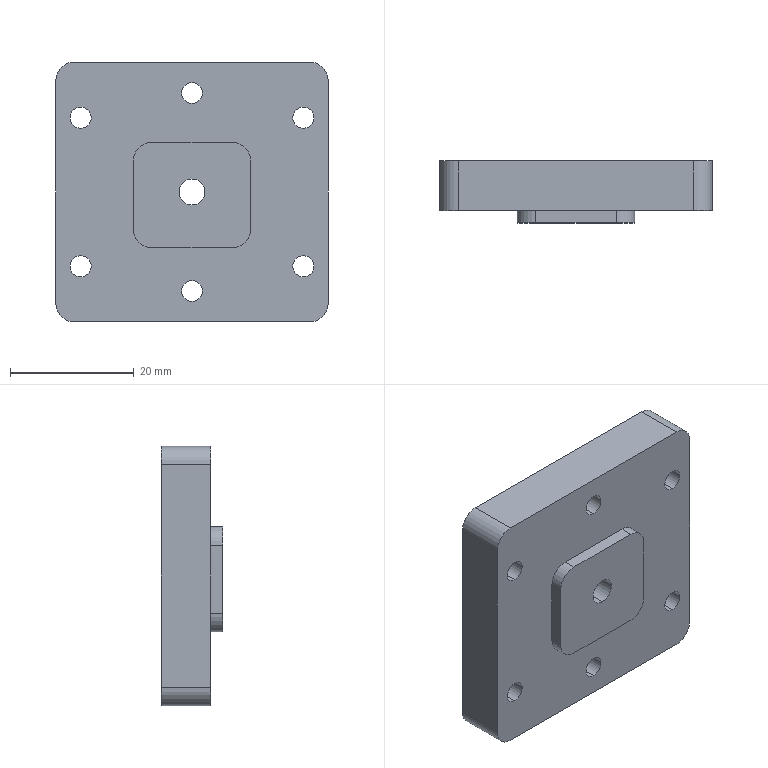Part | STEP file | 10000020483swp000-1 | 1 solid | 51 faces | box 44 x 10 x 42 mm | volume 14387 mm3 | cylinder 34 | plane 17 | commonest cylinder face diameters 6 x20 3.4 x12 4.2 x2
STEP:
#1=CARTESIAN_POINT('',(0.,-2.,-2.1));
#2=VERTEX_POINT('',#1);
#3=CARTESIAN_POINT('',(0.,-2.,2.1));
#4=VERTEX_POINT('',#3);
#5=CARTESIAN_POINT('',(0.,-2.,0.));
#6=DIRECTION('',(0.,1.,0.));
#7=DIRECTION('',(0.,0.,1.));
#8=AXIS2_PLACEMENT_3D('',#5,#6,#7);
#9=CIRCLE('',#8,2.1);
#10=EDGE_CURVE('',#2,#4,#9,.T.);
#11=ORIENTED_EDGE('',*,*,#10,.F.);
#12=CARTESIAN_POINT('',(0.,8.,-2.1));
#13=VERTEX_POINT('',#12);
#14=CARTESIAN_POINT('',(0.,8.,-2.1));
#15=DIRECTION('',(0.,1.,0.));
#16=VECTOR('',#15,1000.);
#17=LINE('',#14,#16);
#18=EDGE_CURVE('',#2,#13,#17,.T.);
#19=ORIENTED_EDGE('',*,*,#18,.T.);
#20=CARTESIAN_POINT('',(0.,8.,2.1));
#21=VERTEX_POINT('',#20);
#22=CARTESIAN_POINT('',(0.,8.,0.));
#23=DIRECTION('',(0.,1.,0.));
#24=DIRECTION('',(0.,0.,1.));
#25=AXIS2_PLACEMENT_3D('',#22,#23,#24);
#26=CIRCLE('',#25,2.1);
#27=EDGE_CURVE('',#13,#21,#26,.T.);
#28=ORIENTED_EDGE('',*,*,#27,.T.);
#29=CARTESIAN_POINT('',(0.,8.,2.1));
#30=DIRECTION('',(0.,1.,0.));
#31=VECTOR('',#30,1000.);
#32=LINE('',#29,#31);
#33=EDGE_CURVE('',#4,#21,#32,.T.);
#34=ORIENTED_EDGE('',*,*,#33,.F.);
#35=EDGE_LOOP('',(#11,#19,#28,#34));
#36=FACE_OUTER_BOUND('',#35,.T.);
#37=CARTESIAN_POINT('',(0.,8.,0.));
#38=DIRECTION('',(0.,1.,0.));
#39=DIRECTION('',(0.,0.,1.));
#40=AXIS2_PLACEMENT_3D('',#37,#38,#39);
#41=CYLINDRICAL_SURFACE('',#40,2.1);
#42=ADVANCED_FACE('',(#36),#41,.F.);
#43=CARTESIAN_POINT('',(0.,4.6,-19.));
#44=VERTEX_POINT('',#43);
#45=CARTESIAN_POINT('',(0.,4.6,-13.));
#46=VERTEX_POINT('',#45);
#47=CARTESIAN_POINT('',(0.,4.6,-16.));
#48=DIRECTION('',(0.,1.,0.));
#49=DIRECTION('',(0.,0.,1.));
#50=AXIS2_PLACEMENT_3D('',#47,#48,#49);
#51=CIRCLE('',#50,3.);
#52=EDGE_CURVE('',#44,#46,#51,.T.);
#53=ORIENTED_EDGE('',*,*,#52,.F.);
#54=CARTESIAN_POINT('',(0.,8.,-19.));
#55=VERTEX_POINT('',#54);
#56=CARTESIAN_POINT('',(0.,8.,-19.));
#57=DIRECTION('',(0.,1.,0.));
#58=VECTOR('',#57,1000.);
#59=LINE('',#56,#58);
#60=EDGE_CURVE('',#44,#55,#59,.T.);
#61=ORIENTED_EDGE('',*,*,#60,.T.);
#62=CARTESIAN_POINT('',(0.,8.,-13.));
#63=VERTEX_POINT('',#62);
#64=CARTESIAN_POINT('',(0.,8.,-16.));
#65=DIRECTION('',(0.,1.,0.));
#66=DIRECTION('',(0.,0.,1.));
#67=AXIS2_PLACEMENT_3D('',#64,#65,#66);
#68=CIRCLE('',#67,3.);
#69=EDGE_CURVE('',#55,#63,#68,.T.);
#70=ORIENTED_EDGE('',*,*,#69,.T.);
#71=CARTESIAN_POINT('',(0.,8.,-13.));
#72=DIRECTION('',(0.,1.,0.));
#73=VECTOR('',#72,1000.);
#74=LINE('',#71,#73);
#75=EDGE_CURVE('',#46,#63,#74,.T.);
#76=ORIENTED_EDGE('',*,*,#75,.F.);
#77=EDGE_LOOP('',(#53,#61,#70,#76));
#78=FACE_OUTER_BOUND('',#77,.T.);
#79=CARTESIAN_POINT('',(0.,8.,-16.));
#80=DIRECTION('',(0.,1.,0.));
#81=DIRECTION('',(0.,0.,1.));
#82=AXIS2_PLACEMENT_3D('',#79,#80,#81);
#83=CYLINDRICAL_SURFACE('',#82,3.);
#84=ADVANCED_FACE('',(#78),#83,.F.);
#85=CARTESIAN_POINT('',(0.,0.,-17.7));
#86=VERTEX_POINT('',#85);
#87=CARTESIAN_POINT('',(0.,0.,-14.3));
#88=VERTEX_POINT('',#87);
#89=CARTESIAN_POINT('',(0.,0.,-16.));
#90=DIRECTION('',(0.,1.,0.));
#91=DIRECTION('',(0.,0.,1.));
#92=AXIS2_PLACEMENT_3D('',#89,#90,#91);
#93=CIRCLE('',#92,1.7);
#94=EDGE_CURVE('',#86,#88,#93,.T.);
#95=ORIENTED_EDGE('',*,*,#94,.F.);
#96=CARTESIAN_POINT('',(0.,4.6,-17.7));
#97=VERTEX_POINT('',#96);
#98=CARTESIAN_POINT('',(0.,8.,-17.7));
#99=DIRECTION('',(0.,1.,0.));
#100=VECTOR('',#99,1000.);
#101=LINE('',#98,#100);
#102=EDGE_CURVE('',#86,#97,#101,.T.);
#103=ORIENTED_EDGE('',*,*,#102,.T.);
#104=CARTESIAN_POINT('',(0.,4.6,-14.3));
#105=VERTEX_POINT('',#104);
#106=CARTESIAN_POINT('',(0.,4.6,-16.));
#107=DIRECTION('',(0.,1.,0.));
#108=DIRECTION('',(0.,0.,1.));
#109=AXIS2_PLACEMENT_3D('',#106,#107,#108);
#110=CIRCLE('',#109,1.7);
#111=EDGE_CURVE('',#97,#105,#110,.T.);
#112=ORIENTED_EDGE('',*,*,#111,.T.);
#113=CARTESIAN_POINT('',(0.,8.,-14.3));
#114=DIRECTION('',(0.,1.,0.));
#115=VECTOR('',#114,1000.);
#116=LINE('',#113,#115);
#117=EDGE_CURVE('',#88,#105,#116,.T.);
#118=ORIENTED_EDGE('',*,*,#117,.F.);
#119=EDGE_LOOP('',(#95,#103,#112,#118));
#120=FACE_OUTER_BOUND('',#119,.T.);
#121=CARTESIAN_POINT('',(0.,8.,-16.));
#122=DIRECTION('',(0.,1.,0.));
#123=DIRECTION('',(0.,0.,1.));
#124=AXIS2_PLACEMENT_3D('',#121,#122,#123);
#125=CYLINDRICAL_SURFACE('',#124,1.7);
#126=ADVANCED_FACE('',(#120),#125,.F.);
#127=CARTESIAN_POINT('',(-18.,4.6,-15.));
#128=VERTEX_POINT('',#127);
#129=CARTESIAN_POINT('',(-18.,4.6,-9.));
#130=VERTEX_POINT('',#129);
#131=CARTESIAN_POINT('',(-18.,4.6,-12.));
#132=DIRECTION('',(0.,1.,0.));
#133=DIRECTION('',(0.,0.,1.));
#134=AXIS2_PLACEMENT_3D('',#131,#132,#133);
#135=CIRCLE('',#134,3.);
#136=EDGE_CURVE('',#128,#130,#135,.T.);
#137=ORIENTED_EDGE('',*,*,#136,.F.);
#138=CARTESIAN_POINT('',(-18.,8.,-15.));
#139=VERTEX_POINT('',#138);
#140=CARTESIAN_POINT('',(-18.,8.,-15.));
#141=DIRECTION('',(0.,1.,0.));
#142=VECTOR('',#141,1000.);
#143=LINE('',#140,#142);
#144=EDGE_CURVE('',#128,#139,#143,.T.);
#145=ORIENTED_EDGE('',*,*,#144,.T.);
#146=CARTESIAN_POINT('',(-18.,8.,-9.));
#147=VERTEX_POINT('',#146);
#148=CARTESIAN_POINT('',(-18.,8.,-12.));
#149=DIRECTION('',(0.,1.,0.));
#150=DIRECTION('',(0.,0.,1.));
#151=AXIS2_PLACEMENT_3D('',#148,#149,#150);
#152=CIRCLE('',#151,3.);
#153=EDGE_CURVE('',#139,#147,#152,.T.);
#154=ORIENTED_EDGE('',*,*,#153,.T.);
#155=CARTESIAN_POINT('',(-18.,8.,-9.));
#156=DIRECTION('',(0.,1.,0.));
#157=VECTOR('',#156,1000.);
#158=LINE('',#155,#157);
#159=EDGE_CURVE('',#130,#147,#158,.T.);
#160=ORIENTED_EDGE('',*,*,#159,.F.);
#161=EDGE_LOOP('',(#137,#145,#154,#160));
#162=FACE_OUTER_BOUND('',#161,.T.);
#163=CARTESIAN_POINT('',(-18.,8.,-12.));
#164=DIRECTION('',(0.,1.,0.));
#165=DIRECTION('',(0.,0.,1.));
#166=AXIS2_PLACEMENT_3D('',#163,#164,#165);
#167=CYLINDRICAL_SURFACE('',#166,3.);
#168=ADVANCED_FACE('',(#162),#167,.F.);
#169=CARTESIAN_POINT('',(-18.,0.,-13.7));
#170=VERTEX_POINT('',#169);
#171=CARTESIAN_POINT('',(-18.,0.,-10.3));
#172=VERTEX_POINT('',#171);
#173=CARTESIAN_POINT('',(-18.,0.,-12.));
#174=DIRECTION('',(0.,1.,0.));
#175=DIRECTION('',(0.,0.,1.));
#176=AXIS2_PLACEMENT_3D('',#173,#174,#175);
#177=CIRCLE('',#176,1.7);
#178=EDGE_CURVE('',#170,#172,#177,.T.);
#179=ORIENTED_EDGE('',*,*,#178,.F.);
#180=CARTESIAN_POINT('',(-18.,4.6,-13.7));
#181=VERTEX_POINT('',#180);
#182=CARTESIAN_POINT('',(-18.,8.,-13.7));
#183=DIRECTION('',(0.,1.,0.));
#184=VECTOR('',#183,1000.);
#185=LINE('',#182,#184);
#186=EDGE_CURVE('',#170,#181,#185,.T.);
#187=ORIENTED_EDGE('',*,*,#186,.T.);
#188=CARTESIAN_POINT('',(-18.,4.6,-10.3));
#189=VERTEX_POINT('',#188);
#190=CARTESIAN_POINT('',(-18.,4.6,-12.));
#191=DIRECTION('',(0.,1.,0.));
#192=DIRECTION('',(0.,0.,1.));
#193=AXIS2_PLACEMENT_3D('',#190,#191,#192);
#194=CIRCLE('',#193,1.7);
#195=EDGE_CURVE('',#181,#189,#194,.T.);
#196=ORIENTED_EDGE('',*,*,#195,.T.);
#197=CARTESIAN_POINT('',(-18.,8.,-10.3));
#198=DIRECTION('',(0.,1.,0.));
#199=VECTOR('',#198,1000.);
#200=LINE('',#197,#199);
#201=EDGE_CURVE('',#172,#189,#200,.T.);
#202=ORIENTED_EDGE('',*,*,#201,.F.);
#203=EDGE_LOOP('',(#179,#187,#196,#202));
#204=FACE_OUTER_BOUND('',#203,.T.);
#205=CARTESIAN_POINT('',(-18.,8.,-12.));
#206=DIRECTION('',(0.,1.,0.));
#207=DIRECTION('',(0.,0.,1.));
#208=AXIS2_PLACEMENT_3D('',#205,#206,#207);
#209=CYLINDRICAL_SURFACE('',#208,1.7);
#210=ADVANCED_FACE('',(#204),#209,.F.);
#211=CARTESIAN_POINT('',(-18.,4.6,9.));
#212=VERTEX_POINT('',#211);
#213=CARTESIAN_POINT('',(-18.,4.6,15.));
#214=VERTEX_POINT('',#213);
#215=CARTESIAN_POINT('',(-18.,4.6,12.));
#216=DIRECTION('',(0.,1.,0.));
#217=DIRECTION('',(0.,0.,1.));
#218=AXIS2_PLACEMENT_3D('',#215,#216,#217);
#219=CIRCLE('',#218,3.);
#220=EDGE_CURVE('',#212,#214,#219,.T.);
#221=ORIENTED_EDGE('',*,*,#220,.F.);
#222=CARTESIAN_POINT('',(-18.,8.,9.));
#223=VERTEX_POINT('',#222);
#224=CARTESIAN_POINT('',(-18.,8.,9.));
#225=DIRECTION('',(0.,1.,0.));
#226=VECTOR('',#225,1000.);
#227=LINE('',#224,#226);
#228=EDGE_CURVE('',#212,#223,#227,.T.);
#229=ORIENTED_EDGE('',*,*,#228,.T.);
#230=CARTESIAN_POINT('',(-18.,8.,15.));
#231=VERTEX_POINT('',#230);
#232=CARTESIAN_POINT('',(-18.,8.,12.));
#233=DIRECTION('',(0.,1.,0.));
#234=DIRECTION('',(0.,0.,1.));
#235=AXIS2_PLACEMENT_3D('',#232,#233,#234);
#236=CIRCLE('',#235,3.);
#237=EDGE_CURVE('',#223,#231,#236,.T.);
#238=ORIENTED_EDGE('',*,*,#237,.T.);
#239=CARTESIAN_POINT('',(-18.,8.,15.));
#240=DIRECTION('',(0.,1.,0.));
#241=VECTOR('',#240,1000.);
#242=LINE('',#239,#241);
#243=EDGE_CURVE('',#214,#231,#242,.T.);
#244=ORIENTED_EDGE('',*,*,#243,.F.);
#245=EDGE_LOOP('',(#221,#229,#238,#244));
#246=FACE_OUTER_BOUND('',#245,.T.);
#247=CARTESIAN_POINT('',(-18.,8.,12.));
#248=DIRECTION('',(0.,1.,0.));
#249=DIRECTION('',(0.,0.,1.));
#250=AXIS2_PLACEMENT_3D('',#247,#248,#249);
#251=CYLINDRICAL_SURFACE('',#250,3.);
#252=ADVANCED_FACE('',(#246),#251,.F.);
#253=CARTESIAN_POINT('',(-18.,0.,10.3));
#254=VERTEX_POINT('',#253);
#255=CARTESIAN_POINT('',(-18.,0.,13.7));
#256=VERTEX_POINT('',#255);
#257=CARTESIAN_POINT('',(-18.,0.,12.));
#258=DIRECTION('',(0.,1.,0.));
#259=DIRECTION('',(0.,0.,1.));
#260=AXIS2_PLACEMENT_3D('',#257,#258,#259);
#261=CIRCLE('',#260,1.7);
#262=EDGE_CURVE('',#254,#256,#261,.T.);
#263=ORIENTED_EDGE('',*,*,#262,.F.);
#264=CARTESIAN_POINT('',(-18.,4.6,10.3));
#265=VERTEX_POINT('',#264);
#266=CARTESIAN_POINT('',(-18.,8.,10.3));
#267=DIRECTION('',(0.,1.,0.));
#268=VECTOR('',#267,1000.);
#269=LINE('',#266,#268);
#270=EDGE_CURVE('',#254,#265,#269,.T.);
#271=ORIENTED_EDGE('',*,*,#270,.T.);
#272=CARTESIAN_POINT('',(-18.,4.6,13.7));
#273=VERTEX_POINT('',#272);
#274=CARTESIAN_POINT('',(-18.,4.6,12.));
#275=DIRECTION('',(0.,1.,0.));
#276=DIRECTION('',(0.,0.,1.));
#277=AXIS2_PLACEMENT_3D('',#274,#275,#276);
#278=CIRCLE('',#277,1.7);
#279=EDGE_CURVE('',#265,#273,#278,.T.);
#280=ORIENTED_EDGE('',*,*,#279,.T.);
#281=CARTESIAN_POINT('',(-18.,8.,13.7));
#282=DIRECTION('',(0.,1.,0.));
#283=VECTOR('',#282,1000.);
#284=LINE('',#281,#283);
#285=EDGE_CURVE('',#256,#273,#284,.T.);
#286=ORIENTED_EDGE('',*,*,#285,.F.);
#287=EDGE_LOOP('',(#263,#271,#280,#286));
#288=FACE_OUTER_BOUND('',#287,.T.);
#289=CARTESIAN_POINT('',(-18.,8.,12.));
#290=DIRECTION('',(0.,1.,0.));
#291=DIRECTION('',(0.,0.,1.));
#292=AXIS2_PLACEMENT_3D('',#289,#290,#291);
#293=CYLINDRICAL_SURFACE('',#292,1.7);
#294=ADVANCED_FACE('',(#288),#293,.F.);
#295=CARTESIAN_POINT('',(0.,4.6,13.));
#296=VERTEX_POINT('',#295);
#297=CARTESIAN_POINT('',(0.,4.6,19.));
#298=VERTEX_POINT('',#297);
#299=CARTESIAN_POINT('',(0.,4.6,16.));
#300=DIRECTION('',(0.,1.,0.));
#301=DIRECTION('',(0.,0.,1.));
#302=AXIS2_PLACEMENT_3D('',#299,#300,#301);
#303=CIRCLE('',#302,3.);
#304=EDGE_CURVE('',#296,#298,#303,.T.);
#305=ORIENTED_EDGE('',*,*,#304,.F.);
#306=CARTESIAN_POINT('',(0.,8.,13.));
#307=VERTEX_POINT('',#306);
#308=CARTESIAN_POINT('',(0.,8.,13.));
#309=DIRECTION('',(0.,1.,0.));
#310=VECTOR('',#309,1000.);
#311=LINE('',#308,#310);
#312=EDGE_CURVE('',#296,#307,#311,.T.);
#313=ORIENTED_EDGE('',*,*,#312,.T.);
#314=CARTESIAN_POINT('',(0.,8.,19.));
#315=VERTEX_POINT('',#314);
#316=CARTESIAN_POINT('',(0.,8.,16.));
#317=DIRECTION('',(0.,1.,0.));
#318=DIRECTION('',(0.,0.,1.));
#319=AXIS2_PLACEMENT_3D('',#316,#317,#318);
#320=CIRCLE('',#319,3.);
#321=EDGE_CURVE('',#307,#315,#320,.T.);
#322=ORIENTED_EDGE('',*,*,#321,.T.);
#323=CARTESIAN_POINT('',(0.,8.,19.));
#324=DIRECTION('',(0.,1.,0.));
#325=VECTOR('',#324,1000.);
#326=LINE('',#323,#325);
#327=EDGE_CURVE('',#298,#315,#326,.T.);
#328=ORIENTED_EDGE('',*,*,#327,.F.);
#329=EDGE_LOOP('',(#305,#313,#322,#328));
#330=FACE_OUTER_BOUND('',#329,.T.);
#331=CARTESIAN_POINT('',(0.,8.,16.));
#332=DIRECTION('',(0.,1.,0.));
#333=DIRECTION('',(0.,0.,1.));
#334=AXIS2_PLACEMENT_3D('',#331,#332,#333);
#335=CYLINDRICAL_SURFACE('',#334,3.);
#336=ADVANCED_FACE('',(#330),#335,.F.);
#337=CARTESIAN_POINT('',(0.,0.,14.3));
#338=VERTEX_POINT('',#337);
#339=CARTESIAN_POINT('',(0.,0.,17.7));
#340=VERTEX_POINT('',#339);
#341=CARTESIAN_POINT('',(0.,0.,16.));
#342=DIRECTION('',(0.,1.,0.));
#343=DIRECTION('',(0.,0.,1.));
#344=AXIS2_PLACEMENT_3D('',#341,#342,#343);
#345=CIRCLE('',#344,1.7);
#346=EDGE_CURVE('',#338,#340,#345,.T.);
#347=ORIENTED_EDGE('',*,*,#346,.F.);
#348=CARTESIAN_POINT('',(0.,4.6,14.3));
#349=VERTEX_POINT('',#348);
#350=CARTESIAN_POINT('',(0.,8.,14.3));
#351=DIRECTION('',(0.,1.,0.));
#352=VECTOR('',#351,1000.);
#353=LINE('',#350,#352);
#354=EDGE_CURVE('',#338,#349,#353,.T.);
#355=ORIENTED_EDGE('',*,*,#354,.T.);
#356=CARTESIAN_POINT('',(0.,4.6,17.7));
#357=VERTEX_POINT('',#356);
#358=CARTESIAN_POINT('',(0.,4.6,16.));
#359=DIRECTION('',(0.,1.,0.));
#360=DIRECTION('',(0.,0.,1.));
#361=AXIS2_PLACEMENT_3D('',#358,#359,#360);
#362=CIRCLE('',#361,1.7);
#363=EDGE_CURVE('',#349,#357,#362,.T.);
#364=ORIENTED_EDGE('',*,*,#363,.T.);
#365=CARTESIAN_POINT('',(0.,8.,17.7));
#366=DIRECTION('',(0.,1.,0.));
#367=VECTOR('',#366,1000.);
#368=LINE('',#365,#367);
#369=EDGE_CURVE('',#340,#357,#368,.T.);
#370=ORIENTED_EDGE('',*,*,#369,.F.);
#371=EDGE_LOOP('',(#347,#355,#364,#370));
#372=FACE_OUTER_BOUND('',#371,.T.);
#373=CARTESIAN_POINT('',(0.,8.,16.));
#374=DIRECTION('',(0.,1.,0.));
#375=DIRECTION('',(0.,0.,1.));
#376=AXIS2_PLACEMENT_3D('',#373,#374,#375);
#377=CYLINDRICAL_SURFACE('',#376,1.7);
#378=ADVANCED_FACE('',(#372),#377,.F.);
#379=CARTESIAN_POINT('',(18.,4.6,9.));
#380=VERTEX_POINT('',#379);
#381=CARTESIAN_POINT('',(18.,4.6,15.));
#382=VERTEX_POINT('',#381);
#383=CARTESIAN_POINT('',(18.,4.6,12.));
#384=DIRECTION('',(0.,1.,0.));
#385=DIRECTION('',(0.,0.,1.));
#386=AXIS2_PLACEMENT_3D('',#383,#384,#385);
#387=CIRCLE('',#386,3.);
#388=EDGE_CURVE('',#380,#382,#387,.T.);
#389=ORIENTED_EDGE('',*,*,#388,.F.);
#390=CARTESIAN_POINT('',(18.,8.,9.));
#391=VERTEX_POINT('',#390);
#392=CARTESIAN_POINT('',(18.,8.,9.));
#393=DIRECTION('',(0.,1.,0.));
#394=VECTOR('',#393,1000.);
#395=LINE('',#392,#394);
#396=EDGE_CURVE('',#380,#391,#395,.T.);
#397=ORIENTED_EDGE('',*,*,#396,.T.);
#398=CARTESIAN_POINT('',(18.,8.,15.));
#399=VERTEX_POINT('',#398);
#400=CARTESIAN_POINT('',(18.,8.,12.));
#401=DIRECTION('',(0.,1.,0.));
#402=DIRECTION('',(0.,0.,1.));
#403=AXIS2_PLACEMENT_3D('',#400,#401,#402);
#404=CIRCLE('',#403,3.);
#405=EDGE_CURVE('',#391,#399,#404,.T.);
#406=ORIENTED_EDGE('',*,*,#405,.T.);
#407=CARTESIAN_POINT('',(18.,8.,15.));
#408=DIRECTION('',(0.,1.,0.));
#409=VECTOR('',#408,1000.);
#410=LINE('',#407,#409);
#411=EDGE_CURVE('',#382,#399,#410,.T.);
#412=ORIENTED_EDGE('',*,*,#411,.F.);
#413=EDGE_LOOP('',(#389,#397,#406,#412));
#414=FACE_OUTER_BOUND('',#413,.T.);
#415=CARTESIAN_POINT('',(18.,8.,12.));
#416=DIRECTION('',(0.,1.,0.));
#417=DIRECTION('',(0.,0.,1.));
#418=AXIS2_PLACEMENT_3D('',#415,#416,#417);
#419=CYLINDRICAL_SURFACE('',#418,3.);
#420=ADVANCED_FACE('',(#414),#419,.F.);
#421=CARTESIAN_POINT('',(18.,0.,10.3));
#422=VERTEX_POINT('',#421);
#423=CARTESIAN_POINT('',(18.,0.,13.7));
#424=VERTEX_POINT('',#423);
#425=CARTESIAN_POINT('',(18.,0.,12.));
#426=DIRECTION('',(0.,1.,0.));
#427=DIRECTION('',(0.,0.,1.));
#428=AXIS2_PLACEMENT_3D('',#425,#426,#427);
#429=CIRCLE('',#428,1.7);
#430=EDGE_CURVE('',#422,#424,#429,.T.);
#431=ORIENTED_EDGE('',*,*,#430,.F.);
#432=CARTESIAN_POINT('',(18.,4.6,10.3));
#433=VERTEX_POINT('',#432);
#434=CARTESIAN_POINT('',(18.,8.,10.3));
#435=DIRECTION('',(0.,1.,0.));
#436=VECTOR('',#435,1000.);
#437=LINE('',#434,#436);
#438=EDGE_CURVE('',#422,#433,#437,.T.);
#439=ORIENTED_EDGE('',*,*,#438,.T.);
#440=CARTESIAN_POINT('',(18.,4.6,13.7));
#441=VERTEX_POINT('',#440);
#442=CARTESIAN_POINT('',(18.,4.6,12.));
#443=DIRECTION('',(0.,1.,0.));
#444=DIRECTION('',(0.,0.,1.));
#445=AXIS2_PLACEMENT_3D('',#442,#443,#444);
#446=CIRCLE('',#445,1.7);
#447=EDGE_CURVE('',#433,#441,#446,.T.);
#448=ORIENTED_EDGE('',*,*,#447,.T.);
#449=CARTESIAN_POINT('',(18.,8.,13.7));
#450=DIRECTION('',(0.,1.,0.));
#451=VECTOR('',#450,1000.);
#452=LINE('',#449,#451);
#453=EDGE_CURVE('',#424,#441,#452,.T.);
#454=ORIENTED_EDGE('',*,*,#453,.F.);
#455=EDGE_LOOP('',(#431,#439,#448,#454));
#456=FACE_OUTER_BOUND('',#455,.T.);
#457=CARTESIAN_POINT('',(18.,8.,12.));
#458=DIRECTION('',(0.,1.,0.));
#459=DIRECTION('',(0.,0.,1.));
#460=AXIS2_PLACEMENT_3D('',#457,#458,#459);
#461=CYLINDRICAL_SURFACE('',#460,1.7);
#462=ADVANCED_FACE('',(#456),#461,.F.);
#463=CARTESIAN_POINT('',(18.,4.6,-15.));
#464=VERTEX_POINT('',#463);
#465=CARTESIAN_POINT('',(18.,4.6,-9.));
#466=VERTEX_POINT('',#465);
#467=CARTESIAN_POINT('',(18.,4.6,-12.));
#468=DIRECTION('',(0.,1.,0.));
#469=DIRECTION('',(0.,0.,1.));
#470=AXIS2_PLACEMENT_3D('',#467,#468,#469);
#471=CIRCLE('',#470,3.);
#472=EDGE_CURVE('',#464,#466,#471,.T.);
#473=ORIENTED_EDGE('',*,*,#472,.F.);
#474=CARTESIAN_POINT('',(18.,8.,-15.));
#475=VERTEX_POINT('',#474);
#476=CARTESIAN_POINT('',(18.,8.,-15.));
#477=DIRECTION('',(0.,1.,0.));
#478=VECTOR('',#477,1000.);
#479=LINE('',#476,#478);
#480=EDGE_CURVE('',#464,#475,#479,.T.);
#481=ORIENTED_EDGE('',*,*,#480,.T.);
#482=CARTESIAN_POINT('',(18.,8.,-9.));
#483=VERTEX_POINT('',#482);
#484=CARTESIAN_POINT('',(18.,8.,-12.));
#485=DIRECTION('',(0.,1.,0.));
#486=DIRECTION('',(0.,0.,1.));
#487=AXIS2_PLACEMENT_3D('',#484,#485,#486);
#488=CIRCLE('',#487,3.);
#489=EDGE_CURVE('',#475,#483,#488,.T.);
#490=ORIENTED_EDGE('',*,*,#489,.T.);
#491=CARTESIAN_POINT('',(18.,8.,-9.));
#492=DIRECTION('',(0.,1.,0.));
#493=VECTOR('',#492,1000.);
#494=LINE('',#491,#493);
#495=EDGE_CURVE('',#466,#483,#494,.T.);
#496=ORIENTED_EDGE('',*,*,#495,.F.);
#497=EDGE_LOOP('',(#473,#481,#490,#496));
#498=FACE_OUTER_BOUND('',#497,.T.);
#499=CARTESIAN_POINT('',(18.,8.,-12.));
#500=DIRECTION('',(0.,1.,0.));
#501=DIRECTION('',(0.,0.,1.));
#502=AXIS2_PLACEMENT_3D('',#499,#500,#501);
#503=CYLINDRICAL_SURFACE('',#502,3.);
#504=ADVANCED_FACE('',(#498),#503,.F.);
#505=CARTESIAN_POINT('',(18.,0.,-13.7));
#506=VERTEX_POINT('',#505);
#507=CARTESIAN_POINT('',(18.,0.,-10.3));
#508=VERTEX_POINT('',#507);
#509=CARTESIAN_POINT('',(18.,0.,-12.));
#510=DIRECTION('',(0.,1.,0.));
#511=DIRECTION('',(0.,0.,1.));
#512=AXIS2_PLACEMENT_3D('',#509,#510,#511);
#513=CIRCLE('',#512,1.7);
#514=EDGE_CURVE('',#506,#508,#513,.T.);
#515=ORIENTED_EDGE('',*,*,#514,.F.);
#516=CARTESIAN_POINT('',(18.,4.6,-13.7));
#517=VERTEX_POINT('',#516);
#518=CARTESIAN_POINT('',(18.,8.,-13.7));
#519=DIRECTION('',(0.,1.,0.));
#520=VECTOR('',#519,1000.);
#521=LINE('',#518,#520);
#522=EDGE_CURVE('',#506,#517,#521,.T.);
#523=ORIENTED_EDGE('',*,*,#522,.T.);
#524=CARTESIAN_POINT('',(18.,4.6,-10.3));
#525=VERTEX_POINT('',#524);
#526=CARTESIAN_POINT('',(18.,4.6,-12.));
#527=DIRECTION('',(0.,1.,0.));
#528=DIRECTION('',(0.,0.,1.));
#529=AXIS2_PLACEMENT_3D('',#526,#527,#528);
#530=CIRCLE('',#529,1.7);
#531=EDGE_CURVE('',#517,#525,#530,.T.);
#532=ORIENTED_EDGE('',*,*,#531,.T.);
#533=CARTESIAN_POINT('',(18.,8.,-10.3));
#534=DIRECTION('',(0.,1.,0.));
#535=VECTOR('',#534,1000.);
#536=LINE('',#533,#535);
#537=EDGE_CURVE('',#508,#525,#536,.T.);
#538=ORIENTED_EDGE('',*,*,#537,.F.);
#539=EDGE_LOOP('',(#515,#523,#532,#538));
#540=FACE_OUTER_BOUND('',#539,.T.);
#541=CARTESIAN_POINT('',(18.,8.,-12.));
#542=DIRECTION('',(0.,1.,0.));
#543=DIRECTION('',(0.,0.,1.));
#544=AXIS2_PLACEMENT_3D('',#541,#542,#543);
#545=CYLINDRICAL_SURFACE('',#544,1.7);
#546=ADVANCED_FACE('',(#540),#545,.F.);
#547=CARTESIAN_POINT('',(0.,0.,-16.));
#548=DIRECTION('',(0.,1.,0.));
#549=DIRECTION('',(0.,0.,1.));
#550=AXIS2_PLACEMENT_3D('',#547,#548,#549);
#551=CIRCLE('',#550,1.7);
#552=EDGE_CURVE('',#88,#86,#551,.T.);
#553=ORIENTED_EDGE('',*,*,#552,.T.);
#554=ORIENTED_EDGE('',*,*,#94,.T.);
#555=EDGE_LOOP('',(#553,#554));
#556=FACE_BOUND('',#555,.T.);
#557=CARTESIAN_POINT('',(-18.,0.,-12.));
#558=DIRECTION('',(0.,1.,0.));
#559=DIRECTION('',(0.,0.,1.));
#560=AXIS2_PLACEMENT_3D('',#557,#558,#559);
#561=CIRCLE('',#560,1.7);
#562=EDGE_CURVE('',#172,#170,#561,.T.);
#563=ORIENTED_EDGE('',*,*,#562,.T.);
#564=ORIENTED_EDGE('',*,*,#178,.T.);
#565=EDGE_LOOP('',(#563,#564));
#566=FACE_BOUND('',#565,.T.);
#567=CARTESIAN_POINT('',(-18.,0.,12.));
#568=DIRECTION('',(0.,1.,0.));
#569=DIRECTION('',(0.,0.,1.));
#570=AXIS2_PLACEMENT_3D('',#567,#568,#569);
#571=CIRCLE('',#570,1.7);
#572=EDGE_CURVE('',#256,#254,#571,.T.);
#573=ORIENTED_EDGE('',*,*,#572,.T.);
#574=ORIENTED_EDGE('',*,*,#262,.T.);
#575=EDGE_LOOP('',(#573,#574));
#576=FACE_BOUND('',#575,.T.);
#577=CARTESIAN_POINT('',(0.,0.,16.));
#578=DIRECTION('',(0.,1.,0.));
#579=DIRECTION('',(0.,0.,1.));
#580=AXIS2_PLACEMENT_3D('',#577,#578,#579);
#581=CIRCLE('',#580,1.7);
#582=EDGE_CURVE('',#340,#338,#581,.T.);
#583=ORIENTED_EDGE('',*,*,#582,.T.);
#584=ORIENTED_EDGE('',*,*,#346,.T.);
#585=EDGE_LOOP('',(#583,#584));
#586=FACE_BOUND('',#585,.T.);
#587=CARTESIAN_POINT('',(18.,0.,12.));
#588=DIRECTION('',(0.,1.,0.));
#589=DIRECTION('',(0.,0.,1.));
#590=AXIS2_PLACEMENT_3D('',#587,#588,#589);
#591=CIRCLE('',#590,1.7);
#592=EDGE_CURVE('',#424,#422,#591,.T.);
#593=ORIENTED_EDGE('',*,*,#592,.T.);
#594=ORIENTED_EDGE('',*,*,#430,.T.);
#595=EDGE_LOOP('',(#593,#594));
#596=FACE_BOUND('',#595,.T.);
#597=CARTESIAN_POINT('',(18.,0.,-12.));
#598=DIRECTION('',(0.,1.,0.));
#599=DIRECTION('',(0.,0.,1.));
#600=AXIS2_PLACEMENT_3D('',#597,#598,#599);
#601=CIRCLE('',#600,1.7);
#602=EDGE_CURVE('',#508,#506,#601,.T.);
#603=ORIENTED_EDGE('',*,*,#602,.T.);
#604=ORIENTED_EDGE('',*,*,#514,.T.);
#605=EDGE_LOOP('',(#603,#604));
#606=FACE_BOUND('',#605,.T.);
#607=CARTESIAN_POINT('',(22.,0.,18.));
#608=VERTEX_POINT('',#607);
#609=CARTESIAN_POINT('',(22.,0.,-18.));
#610=VERTEX_POINT('',#609);
#611=CARTESIAN_POINT('',(22.,0.,-21.));
#612=DIRECTION('',(0.,0.,-1.));
#613=VECTOR('',#612,1000.);
#614=LINE('',#611,#613);
#615=EDGE_CURVE('',#608,#610,#614,.T.);
#616=ORIENTED_EDGE('',*,*,#615,.F.);
#617=CARTESIAN_POINT('',(19.,0.,21.));
#618=VERTEX_POINT('',#617);
#619=CARTESIAN_POINT('',(19.,0.,18.));
#620=DIRECTION('',(0.,-1.,0.));
#621=DIRECTION('',(0.,0.,1.));
#622=AXIS2_PLACEMENT_3D('',#619,#620,#621);
#623=CIRCLE('',#622,3.);
#624=EDGE_CURVE('',#608,#618,#623,.T.);
#625=ORIENTED_EDGE('',*,*,#624,.T.);
#626=CARTESIAN_POINT('',(-19.,0.,21.));
#627=VERTEX_POINT('',#626);
#628=CARTESIAN_POINT('',(-22.,0.,21.));
#629=DIRECTION('',(1.,0.,0.));
#630=VECTOR('',#629,1000.);
#631=LINE('',#628,#630);
#632=EDGE_CURVE('',#627,#618,#631,.T.);
#633=ORIENTED_EDGE('',*,*,#632,.F.);
#634=CARTESIAN_POINT('',(-22.,0.,18.));
#635=VERTEX_POINT('',#634);
#636=CARTESIAN_POINT('',(-19.,0.,18.));
#637=DIRECTION('',(0.,-1.,0.));
#638=DIRECTION('',(0.,0.,1.));
#639=AXIS2_PLACEMENT_3D('',#636,#637,#638);
#640=CIRCLE('',#639,3.);
#641=EDGE_CURVE('',#627,#635,#640,.T.);
#642=ORIENTED_EDGE('',*,*,#641,.T.);
#643=CARTESIAN_POINT('',(-22.,0.,-18.));
#644=VERTEX_POINT('',#643);
#645=CARTESIAN_POINT('',(-22.,0.,-21.));
#646=DIRECTION('',(0.,0.,1.));
#647=VECTOR('',#646,1000.);
#648=LINE('',#645,#647);
#649=EDGE_CURVE('',#644,#635,#648,.T.);
#650=ORIENTED_EDGE('',*,*,#649,.F.);
#651=CARTESIAN_POINT('',(-19.,0.,-21.));
#652=VERTEX_POINT('',#651);
#653=CARTESIAN_POINT('',(-19.,0.,-18.));
#654=DIRECTION('',(0.,-1.,0.));
#655=DIRECTION('',(0.,0.,1.));
#656=AXIS2_PLACEMENT_3D('',#653,#654,#655);
#657=CIRCLE('',#656,3.);
#658=EDGE_CURVE('',#644,#652,#657,.T.);
#659=ORIENTED_EDGE('',*,*,#658,.T.);
#660=CARTESIAN_POINT('',(19.,0.,-21.));
#661=VERTEX_POINT('',#660);
#662=CARTESIAN_POINT('',(-22.,0.,-21.));
#663=DIRECTION('',(-1.,0.,0.));
#664=VECTOR('',#663,1000.);
#665=LINE('',#662,#664);
#666=EDGE_CURVE('',#661,#652,#665,.T.);
#667=ORIENTED_EDGE('',*,*,#666,.F.);
#668=CARTESIAN_POINT('',(19.,0.,-18.));
#669=DIRECTION('',(0.,-1.,0.));
#670=DIRECTION('',(0.,0.,1.));
#671=AXIS2_PLACEMENT_3D('',#668,#669,#670);
#672=CIRCLE('',#671,3.);
#673=EDGE_CURVE('',#661,#610,#672,.T.);
#674=ORIENTED_EDGE('',*,*,#673,.T.);
#675=EDGE_LOOP('',(#616,#625,#633,#642,#650,#659,#667,#674));
#676=FACE_OUTER_BOUND('',#675,.T.);
#677=CARTESIAN_POINT('',(9.5,0.,-6.));
#678=VERTEX_POINT('',#677);
#679=CARTESIAN_POINT('',(9.5,0.,5.));
#680=VERTEX_POINT('',#679);
#681=CARTESIAN_POINT('',(9.5,0.,8.));
#682=DIRECTION('',(0.,0.,1.));
#683=VECTOR('',#682,1000.);
#684=LINE('',#681,#683);
#685=EDGE_CURVE('',#678,#680,#684,.T.);
#686=ORIENTED_EDGE('',*,*,#685,.F.);
#687=CARTESIAN_POINT('',(6.5,0.,-9.));
#688=VERTEX_POINT('',#687);
#689=CARTESIAN_POINT('',(6.5,0.,-6.));
#690=DIRECTION('',(0.,1.,0.));
#691=DIRECTION('',(0.,0.,1.));
#692=AXIS2_PLACEMENT_3D('',#689,#690,#691);
#693=CIRCLE('',#692,3.);
#694=EDGE_CURVE('',#678,#688,#693,.T.);
#695=ORIENTED_EDGE('',*,*,#694,.T.);
#696=CARTESIAN_POINT('',(-6.5,0.,-9.));
#697=VERTEX_POINT('',#696);
#698=CARTESIAN_POINT('',(-9.5,0.,-9.));
#699=DIRECTION('',(1.,0.,0.));
#700=VECTOR('',#699,1000.);
#701=LINE('',#698,#700);
#702=EDGE_CURVE('',#697,#688,#701,.T.);
#703=ORIENTED_EDGE('',*,*,#702,.F.);
#704=CARTESIAN_POINT('',(-9.5,0.,-6.));
#705=VERTEX_POINT('',#704);
#706=CARTESIAN_POINT('',(-6.5,0.,-6.));
#707=DIRECTION('',(0.,1.,0.));
#708=DIRECTION('',(0.,0.,1.));
#709=AXIS2_PLACEMENT_3D('',#706,#707,#708);
#710=CIRCLE('',#709,3.);
#711=EDGE_CURVE('',#697,#705,#710,.T.);
#712=ORIENTED_EDGE('',*,*,#711,.T.);
#713=CARTESIAN_POINT('',(-9.5,0.,5.));
#714=VERTEX_POINT('',#713);
#715=CARTESIAN_POINT('',(-9.5,0.,8.));
#716=DIRECTION('',(0.,0.,-1.));
#717=VECTOR('',#716,1000.);
#718=LINE('',#715,#717);
#719=EDGE_CURVE('',#714,#705,#718,.T.);
#720=ORIENTED_EDGE('',*,*,#719,.F.);
#721=CARTESIAN_POINT('',(-6.5,0.,8.));
#722=VERTEX_POINT('',#721);
#723=CARTESIAN_POINT('',(-6.5,0.,5.));
#724=DIRECTION('',(0.,1.,0.));
#725=DIRECTION('',(0.,0.,1.));
#726=AXIS2_PLACEMENT_3D('',#723,#724,#725);
#727=CIRCLE('',#726,3.);
#728=EDGE_CURVE('',#714,#722,#727,.T.);
#729=ORIENTED_EDGE('',*,*,#728,.T.);
#730=CARTESIAN_POINT('',(6.5,0.,8.));
#731=VERTEX_POINT('',#730);
#732=CARTESIAN_POINT('',(-9.5,0.,8.));
#733=DIRECTION('',(-1.,0.,0.));
#734=VECTOR('',#733,1000.);
#735=LINE('',#732,#734);
#736=EDGE_CURVE('',#731,#722,#735,.T.);
#737=ORIENTED_EDGE('',*,*,#736,.F.);
#738=CARTESIAN_POINT('',(6.5,0.,5.));
#739=DIRECTION('',(0.,1.,0.));
#740=DIRECTION('',(0.,0.,1.));
#741=AXIS2_PLACEMENT_3D('',#738,#739,#740);
#742=CIRCLE('',#741,3.);
#743=EDGE_CURVE('',#731,#680,#742,.T.);
#744=ORIENTED_EDGE('',*,*,#743,.T.);
#745=EDGE_LOOP('',(#686,#695,#703,#712,#720,#729,#737,#744));
#746=FACE_BOUND('',#745,.T.);
#747=CARTESIAN_POINT('',(0.,0.,0.));
#748=DIRECTION('',(0.,1.,0.));
#749=DIRECTION('',(0.,0.,1.));
#750=AXIS2_PLACEMENT_3D('',#747,#748,#749);
#751=PLANE('',#750);
#752=ADVANCED_FACE('',(#556,#566,#576,#586,#596,#606,#676,#746),#751,.F.);
#753=CARTESIAN_POINT('',(22.,8.,18.));
#754=VERTEX_POINT('',#753);
#755=CARTESIAN_POINT('',(22.,8.,-18.));
#756=VERTEX_POINT('',#755);
#757=CARTESIAN_POINT('',(22.,8.,-21.));
#758=DIRECTION('',(0.,0.,-1.));
#759=VECTOR('',#758,1000.);
#760=LINE('',#757,#759);
#761=EDGE_CURVE('',#754,#756,#760,.T.);
#762=ORIENTED_EDGE('',*,*,#761,.F.);
#763=CARTESIAN_POINT('',(22.,8.,18.));
#764=DIRECTION('',(0.,-1.,0.));
#765=VECTOR('',#764,1000.);
#766=LINE('',#763,#765);
#767=EDGE_CURVE('',#754,#608,#766,.T.);
#768=ORIENTED_EDGE('',*,*,#767,.T.);
#769=ORIENTED_EDGE('',*,*,#615,.T.);
#770=CARTESIAN_POINT('',(22.,8.,-18.));
#771=DIRECTION('',(0.,1.,0.));
#772=VECTOR('',#771,1000.);
#773=LINE('',#770,#772);
#774=EDGE_CURVE('',#610,#756,#773,.T.);
#775=ORIENTED_EDGE('',*,*,#774,.T.);
#776=EDGE_LOOP('',(#762,#768,#769,#775));
#777=FACE_OUTER_BOUND('',#776,.T.);
#778=CARTESIAN_POINT('',(22.,8.,-21.));
#779=DIRECTION('',(-1.,0.,0.));
#780=DIRECTION('',(0.,0.,1.));
#781=AXIS2_PLACEMENT_3D('',#778,#779,#780);
#782=PLANE('',#781);
#783=ADVANCED_FACE('',(#777),#782,.F.);
#784=CARTESIAN_POINT('',(19.,8.,-21.));
#785=VERTEX_POINT('',#784);
#786=CARTESIAN_POINT('',(-19.,8.,-21.));
#787=VERTEX_POINT('',#786);
#788=CARTESIAN_POINT('',(-22.,8.,-21.));
#789=DIRECTION('',(-1.,0.,0.));
#790=VECTOR('',#789,1000.);
#791=LINE('',#788,#790);
#792=EDGE_CURVE('',#785,#787,#791,.T.);
#793=ORIENTED_EDGE('',*,*,#792,.F.);
#794=CARTESIAN_POINT('',(19.,8.,-21.));
#795=DIRECTION('',(0.,-1.,0.));
#796=VECTOR('',#795,1000.);
#797=LINE('',#794,#796);
#798=EDGE_CURVE('',#785,#661,#797,.T.);
#799=ORIENTED_EDGE('',*,*,#798,.T.);
#800=ORIENTED_EDGE('',*,*,#666,.T.);
#801=CARTESIAN_POINT('',(-19.,8.,-21.));
#802=DIRECTION('',(0.,1.,0.));
#803=VECTOR('',#802,1000.);
#804=LINE('',#801,#803);
#805=EDGE_CURVE('',#652,#787,#804,.T.);
#806=ORIENTED_EDGE('',*,*,#805,.T.);
#807=EDGE_LOOP('',(#793,#799,#800,#806));
#808=FACE_OUTER_BOUND('',#807,.T.);
#809=CARTESIAN_POINT('',(-22.,8.,-21.));
#810=DIRECTION('',(0.,0.,1.));
#811=DIRECTION('',(1.,0.,0.));
#812=AXIS2_PLACEMENT_3D('',#809,#810,#811);
#813=PLANE('',#812);
#814=ADVANCED_FACE('',(#808),#813,.F.);
#815=ORIENTED_EDGE('',*,*,#649,.T.);
#816=CARTESIAN_POINT('',(-22.,8.,18.));
#817=VERTEX_POINT('',#816);
#818=CARTESIAN_POINT('',(-22.,8.,18.));
#819=DIRECTION('',(0.,1.,0.));
#820=VECTOR('',#819,1000.);
#821=LINE('',#818,#820);
#822=EDGE_CURVE('',#635,#817,#821,.T.);
#823=ORIENTED_EDGE('',*,*,#822,.T.);
#824=CARTESIAN_POINT('',(-22.,8.,-18.));
#825=VERTEX_POINT('',#824);
#826=CARTESIAN_POINT('',(-22.,8.,-21.));
#827=DIRECTION('',(0.,0.,1.));
#828=VECTOR('',#827,1000.);
#829=LINE('',#826,#828);
#830=EDGE_CURVE('',#825,#817,#829,.T.);
#831=ORIENTED_EDGE('',*,*,#830,.F.);
#832=CARTESIAN_POINT('',(-22.,8.,-18.));
#833=DIRECTION('',(0.,-1.,0.));
#834=VECTOR('',#833,1000.);
#835=LINE('',#832,#834);
#836=EDGE_CURVE('',#825,#644,#835,.T.);
#837=ORIENTED_EDGE('',*,*,#836,.T.);
#838=EDGE_LOOP('',(#815,#823,#831,#837));
#839=FACE_OUTER_BOUND('',#838,.T.);
#840=CARTESIAN_POINT('',(-22.,8.,-21.));
#841=DIRECTION('',(1.,0.,0.));
#842=DIRECTION('',(0.,0.,-1.));
#843=AXIS2_PLACEMENT_3D('',#840,#841,#842);
#844=PLANE('',#843);
#845=ADVANCED_FACE('',(#839),#844,.F.);
#846=ORIENTED_EDGE('',*,*,#632,.T.);
#847=CARTESIAN_POINT('',(19.,8.,21.));
#848=VERTEX_POINT('',#847);
#849=CARTESIAN_POINT('',(19.,8.,21.));
#850=DIRECTION('',(0.,1.,0.));
#851=VECTOR('',#850,1000.);
#852=LINE('',#849,#851);
#853=EDGE_CURVE('',#618,#848,#852,.T.);
#854=ORIENTED_EDGE('',*,*,#853,.T.);
#855=CARTESIAN_POINT('',(-19.,8.,21.));
#856=VERTEX_POINT('',#855);
#857=CARTESIAN_POINT('',(-22.,8.,21.));
#858=DIRECTION('',(1.,0.,0.));
#859=VECTOR('',#858,1000.);
#860=LINE('',#857,#859);
#861=EDGE_CURVE('',#856,#848,#860,.T.);
#862=ORIENTED_EDGE('',*,*,#861,.F.);
#863=CARTESIAN_POINT('',(-19.,8.,21.));
#864=DIRECTION('',(0.,-1.,0.));
#865=VECTOR('',#864,1000.);
#866=LINE('',#863,#865);
#867=EDGE_CURVE('',#856,#627,#866,.T.);
#868=ORIENTED_EDGE('',*,*,#867,.T.);
#869=EDGE_LOOP('',(#846,#854,#862,#868));
#870=FACE_OUTER_BOUND('',#869,.T.);
#871=CARTESIAN_POINT('',(-22.,8.,21.));
#872=DIRECTION('',(0.,0.,-1.));
#873=DIRECTION('',(-1.,0.,0.));
#874=AXIS2_PLACEMENT_3D('',#871,#872,#873);
#875=PLANE('',#874);
#876=ADVANCED_FACE('',(#870),#875,.F.);
#877=CARTESIAN_POINT('',(0.,8.,0.));
#878=DIRECTION('',(0.,1.,0.));
#879=DIRECTION('',(0.,0.,1.));
#880=AXIS2_PLACEMENT_3D('',#877,#878,#879);
#881=CIRCLE('',#880,2.1);
#882=EDGE_CURVE('',#21,#13,#881,.T.);
#883=ORIENTED_EDGE('',*,*,#882,.F.);
#884=ORIENTED_EDGE('',*,*,#27,.F.);
#885=EDGE_LOOP('',(#883,#884));
#886=FACE_BOUND('',#885,.T.);
#887=CARTESIAN_POINT('',(0.,8.,-16.));
#888=DIRECTION('',(0.,1.,0.));
#889=DIRECTION('',(0.,0.,1.));
#890=AXIS2_PLACEMENT_3D('',#887,#888,#889);
#891=CIRCLE('',#890,3.);
#892=EDGE_CURVE('',#63,#55,#891,.T.);
#893=ORIENTED_EDGE('',*,*,#892,.F.);
#894=ORIENTED_EDGE('',*,*,#69,.F.);
#895=EDGE_LOOP('',(#893,#894));
#896=FACE_BOUND('',#895,.T.);
#897=CARTESIAN_POINT('',(-18.,8.,-12.));
#898=DIRECTION('',(0.,1.,0.));
#899=DIRECTION('',(0.,0.,1.));
#900=AXIS2_PLACEMENT_3D('',#897,#898,#899);
#901=CIRCLE('',#900,3.);
#902=EDGE_CURVE('',#147,#139,#901,.T.);
#903=ORIENTED_EDGE('',*,*,#902,.F.);
#904=ORIENTED_EDGE('',*,*,#153,.F.);
#905=EDGE_LOOP('',(#903,#904));
#906=FACE_BOUND('',#905,.T.);
#907=CARTESIAN_POINT('',(-18.,8.,12.));
#908=DIRECTION('',(0.,1.,0.));
#909=DIRECTION('',(0.,0.,1.));
#910=AXIS2_PLACEMENT_3D('',#907,#908,#909);
#911=CIRCLE('',#910,3.);
#912=EDGE_CURVE('',#231,#223,#911,.T.);
#913=ORIENTED_EDGE('',*,*,#912,.F.);
#914=ORIENTED_EDGE('',*,*,#237,.F.);
#915=EDGE_LOOP('',(#913,#914));
#916=FACE_BOUND('',#915,.T.);
#917=CARTESIAN_POINT('',(0.,8.,16.));
#918=DIRECTION('',(0.,1.,0.));
#919=DIRECTION('',(0.,0.,1.));
#920=AXIS2_PLACEMENT_3D('',#917,#918,#919);
#921=CIRCLE('',#920,3.);
#922=EDGE_CURVE('',#315,#307,#921,.T.);
#923=ORIENTED_EDGE('',*,*,#922,.F.);
#924=ORIENTED_EDGE('',*,*,#321,.F.);
#925=EDGE_LOOP('',(#923,#924));
#926=FACE_BOUND('',#925,.T.);
#927=CARTESIAN_POINT('',(18.,8.,12.));
#928=DIRECTION('',(0.,1.,0.));
#929=DIRECTION('',(0.,0.,1.));
#930=AXIS2_PLACEMENT_3D('',#927,#928,#929);
#931=CIRCLE('',#930,3.);
#932=EDGE_CURVE('',#399,#391,#931,.T.);
#933=ORIENTED_EDGE('',*,*,#932,.F.);
#934=ORIENTED_EDGE('',*,*,#405,.F.);
#935=EDGE_LOOP('',(#933,#934));
#936=FACE_BOUND('',#935,.T.);
#937=CARTESIAN_POINT('',(18.,8.,-12.));
#938=DIRECTION('',(0.,1.,0.));
#939=DIRECTION('',(0.,0.,1.));
#940=AXIS2_PLACEMENT_3D('',#937,#938,#939);
#941=CIRCLE('',#940,3.);
#942=EDGE_CURVE('',#483,#475,#941,.T.);
#943=ORIENTED_EDGE('',*,*,#942,.F.);
#944=ORIENTED_EDGE('',*,*,#489,.F.);
#945=EDGE_LOOP('',(#943,#944));
#946=FACE_BOUND('',#945,.T.);
#947=ORIENTED_EDGE('',*,*,#861,.T.);
#948=CARTESIAN_POINT('',(19.,8.,18.));
#949=DIRECTION('',(0.,1.,0.));
#950=DIRECTION('',(0.,0.,1.));
#951=AXIS2_PLACEMENT_3D('',#948,#949,#950);
#952=CIRCLE('',#951,3.);
#953=EDGE_CURVE('',#848,#754,#952,.T.);
#954=ORIENTED_EDGE('',*,*,#953,.T.);
#955=ORIENTED_EDGE('',*,*,#761,.T.);
#956=CARTESIAN_POINT('',(19.,8.,-18.));
#957=DIRECTION('',(0.,1.,0.));
#958=DIRECTION('',(0.,0.,1.));
#959=AXIS2_PLACEMENT_3D('',#956,#957,#958);
#960=CIRCLE('',#959,3.);
#961=EDGE_CURVE('',#756,#785,#960,.T.);
#962=ORIENTED_EDGE('',*,*,#961,.T.);
#963=ORIENTED_EDGE('',*,*,#792,.T.);
#964=CARTESIAN_POINT('',(-19.,8.,-18.));
#965=DIRECTION('',(0.,1.,0.));
#966=DIRECTION('',(0.,0.,1.));
#967=AXIS2_PLACEMENT_3D('',#964,#965,#966);
#968=CIRCLE('',#967,3.);
#969=EDGE_CURVE('',#787,#825,#968,.T.);
#970=ORIENTED_EDGE('',*,*,#969,.T.);
#971=ORIENTED_EDGE('',*,*,#830,.T.);
#972=CARTESIAN_POINT('',(-19.,8.,18.));
#973=DIRECTION('',(0.,1.,0.));
#974=DIRECTION('',(0.,0.,1.));
#975=AXIS2_PLACEMENT_3D('',#972,#973,#974);
#976=CIRCLE('',#975,3.);
#977=EDGE_CURVE('',#817,#856,#976,.T.);
#978=ORIENTED_EDGE('',*,*,#977,.T.);
#979=EDGE_LOOP('',(#947,#954,#955,#962,#963,#970,#971,#978));
#980=FACE_OUTER_BOUND('',#979,.T.);
#981=CARTESIAN_POINT('',(0.,8.,0.));
#982=DIRECTION('',(0.,1.,0.));
#983=DIRECTION('',(0.,0.,1.));
#984=AXIS2_PLACEMENT_3D('',#981,#982,#983);
#985=PLANE('',#984);
#986=ADVANCED_FACE('',(#886,#896,#906,#916,#926,#936,#946,#980),#985,.T.);
#987=CARTESIAN_POINT('',(9.5,-2.,-6.));
#988=VERTEX_POINT('',#987);
#989=CARTESIAN_POINT('',(9.5,-2.,5.));
#990=VERTEX_POINT('',#989);
#991=CARTESIAN_POINT('',(9.5,-2.,8.));
#992=DIRECTION('',(0.,0.,1.));
#993=VECTOR('',#992,1000.);
#994=LINE('',#991,#993);
#995=EDGE_CURVE('',#988,#990,#994,.T.);
#996=ORIENTED_EDGE('',*,*,#995,.F.);
#997=CARTESIAN_POINT('',(9.5,-2.,-6.));
#998=DIRECTION('',(0.,1.,0.));
#999=VECTOR('',#998,1000.);
#1000=LINE('',#997,#999);
#1001=EDGE_CURVE('',#988,#678,#1000,.T.);
#1002=ORIENTED_EDGE('',*,*,#1001,.T.);
#1003=ORIENTED_EDGE('',*,*,#685,.T.);
#1004=CARTESIAN_POINT('',(9.5,-2.,5.));
#1005=DIRECTION('',(0.,-1.,0.));
#1006=VECTOR('',#1005,1000.);
#1007=LINE('',#1004,#1006);
#1008=EDGE_CURVE('',#680,#990,#1007,.T.);
#1009=ORIENTED_EDGE('',*,*,#1008,.T.);
#1010=EDGE_LOOP('',(#996,#1002,#1003,#1009));
#1011=FACE_OUTER_BOUND('',#1010,.T.);
#1012=CARTESIAN_POINT('',(9.5,-2.,8.));
#1013=DIRECTION('',(-1.,0.,0.));
#1014=DIRECTION('',(0.,0.,1.));
#1015=AXIS2_PLACEMENT_3D('',#1012,#1013,#1014);
#1016=PLANE('',#1015);
#1017=ADVANCED_FACE('',(#1011),#1016,.F.);
#1018=CARTESIAN_POINT('',(6.5,-2.,8.));
#1019=VERTEX_POINT('',#1018);
#1020=CARTESIAN_POINT('',(-6.5,-2.,8.));
#1021=VERTEX_POINT('',#1020);
#1022=CARTESIAN_POINT('',(-9.5,-2.,8.));
#1023=DIRECTION('',(-1.,0.,0.));
#1024=VECTOR('',#1023,1000.);
#1025=LINE('',#1022,#1024);
#1026=EDGE_CURVE('',#1019,#1021,#1025,.T.);
#1027=ORIENTED_EDGE('',*,*,#1026,.F.);
#1028=CARTESIAN_POINT('',(6.5,-2.,8.));
#1029=DIRECTION('',(0.,1.,0.));
#1030=VECTOR('',#1029,1000.);
#1031=LINE('',#1028,#1030);
#1032=EDGE_CURVE('',#1019,#731,#1031,.T.);
#1033=ORIENTED_EDGE('',*,*,#1032,.T.);
#1034=ORIENTED_EDGE('',*,*,#736,.T.);
#1035=CARTESIAN_POINT('',(-6.5,-2.,8.));
#1036=DIRECTION('',(0.,-1.,0.));
#1037=VECTOR('',#1036,1000.);
#1038=LINE('',#1035,#1037);
#1039=EDGE_CURVE('',#722,#1021,#1038,.T.);
#1040=ORIENTED_EDGE('',*,*,#1039,.T.);
#1041=EDGE_LOOP('',(#1027,#1033,#1034,#1040));
#1042=FACE_OUTER_BOUND('',#1041,.T.);
#1043=CARTESIAN_POINT('',(-9.5,-2.,8.));
#1044=DIRECTION('',(0.,0.,-1.));
#1045=DIRECTION('',(-1.,0.,0.));
#1046=AXIS2_PLACEMENT_3D('',#1043,#1044,#1045);
#1047=PLANE('',#1046);
#1048=ADVANCED_FACE('',(#1042),#1047,.F.);
#1049=ORIENTED_EDGE('',*,*,#719,.T.);
#1050=CARTESIAN_POINT('',(-9.5,-2.,-6.));
#1051=VERTEX_POINT('',#1050);
#1052=CARTESIAN_POINT('',(-9.5,-2.,-6.));
#1053=DIRECTION('',(0.,-1.,0.));
#1054=VECTOR('',#1053,1000.);
#1055=LINE('',#1052,#1054);
#1056=EDGE_CURVE('',#705,#1051,#1055,.T.);
#1057=ORIENTED_EDGE('',*,*,#1056,.T.);
#1058=CARTESIAN_POINT('',(-9.5,-2.,5.));
#1059=VERTEX_POINT('',#1058);
#1060=CARTESIAN_POINT('',(-9.5,-2.,8.));
#1061=DIRECTION('',(0.,0.,-1.));
#1062=VECTOR('',#1061,1000.);
#1063=LINE('',#1060,#1062);
#1064=EDGE_CURVE('',#1059,#1051,#1063,.T.);
#1065=ORIENTED_EDGE('',*,*,#1064,.F.);
#1066=CARTESIAN_POINT('',(-9.5,-2.,5.));
#1067=DIRECTION('',(0.,1.,0.));
#1068=VECTOR('',#1067,1000.);
#1069=LINE('',#1066,#1068);
#1070=EDGE_CURVE('',#1059,#714,#1069,.T.);
#1071=ORIENTED_EDGE('',*,*,#1070,.T.);
#1072=EDGE_LOOP('',(#1049,#1057,#1065,#1071));
#1073=FACE_OUTER_BOUND('',#1072,.T.);
#1074=CARTESIAN_POINT('',(-9.5,-2.,8.));
#1075=DIRECTION('',(1.,0.,0.));
#1076=DIRECTION('',(0.,0.,-1.));
#1077=AXIS2_PLACEMENT_3D('',#1074,#1075,#1076);
#1078=PLANE('',#1077);
#1079=ADVANCED_FACE('',(#1073),#1078,.F.);
#1080=CARTESIAN_POINT('',(-6.5,-2.,-9.));
#1081=VERTEX_POINT('',#1080);
#1082=CARTESIAN_POINT('',(6.5,-2.,-9.));
#1083=VERTEX_POINT('',#1082);
#1084=CARTESIAN_POINT('',(-9.5,-2.,-9.));
#1085=DIRECTION('',(1.,0.,0.));
#1086=VECTOR('',#1085,1000.);
#1087=LINE('',#1084,#1086);
#1088=EDGE_CURVE('',#1081,#1083,#1087,.T.);
#1089=ORIENTED_EDGE('',*,*,#1088,.F.);
#1090=CARTESIAN_POINT('',(-6.5,-2.,-9.));
#1091=DIRECTION('',(0.,1.,0.));
#1092=VECTOR('',#1091,1000.);
#1093=LINE('',#1090,#1092);
#1094=EDGE_CURVE('',#1081,#697,#1093,.T.);
#1095=ORIENTED_EDGE('',*,*,#1094,.T.);
#1096=ORIENTED_EDGE('',*,*,#702,.T.);
#1097=CARTESIAN_POINT('',(6.5,-2.,-9.));
#1098=DIRECTION('',(0.,-1.,0.));
#1099=VECTOR('',#1098,1000.);
#1100=LINE('',#1097,#1099);
#1101=EDGE_CURVE('',#688,#1083,#1100,.T.);
#1102=ORIENTED_EDGE('',*,*,#1101,.T.);
#1103=EDGE_LOOP('',(#1089,#1095,#1096,#1102));
#1104=FACE_OUTER_BOUND('',#1103,.T.);
#1105=CARTESIAN_POINT('',(-9.5,-2.,-9.));
#1106=DIRECTION('',(0.,0.,1.));
#1107=DIRECTION('',(1.,0.,0.));
#1108=AXIS2_PLACEMENT_3D('',#1105,#1106,#1107);
#1109=PLANE('',#1108);
#1110=ADVANCED_FACE('',(#1104),#1109,.F.);
#1111=CARTESIAN_POINT('',(0.,-2.,0.));
#1112=DIRECTION('',(0.,1.,0.));
#1113=DIRECTION('',(0.,0.,1.));
#1114=AXIS2_PLACEMENT_3D('',#1111,#1112,#1113);
#1115=CIRCLE('',#1114,2.1);
#1116=EDGE_CURVE('',#4,#2,#1115,.T.);
#1117=ORIENTED_EDGE('',*,*,#1116,.T.);
#1118=ORIENTED_EDGE('',*,*,#10,.T.);
#1119=EDGE_LOOP('',(#1117,#1118));
#1120=FACE_BOUND('',#1119,.T.);
#1121=ORIENTED_EDGE('',*,*,#1064,.T.);
#1122=CARTESIAN_POINT('',(-6.5,-2.,-6.));
#1123=DIRECTION('',(0.,-1.,0.));
#1124=DIRECTION('',(0.,0.,-1.));
#1125=AXIS2_PLACEMENT_3D('',#1122,#1123,#1124);
#1126=CIRCLE('',#1125,3.);
#1127=EDGE_CURVE('',#1051,#1081,#1126,.T.);
#1128=ORIENTED_EDGE('',*,*,#1127,.T.);
#1129=ORIENTED_EDGE('',*,*,#1088,.T.);
#1130=CARTESIAN_POINT('',(6.5,-2.,-6.));
#1131=DIRECTION('',(0.,-1.,0.));
#1132=DIRECTION('',(0.,0.,-1.));
#1133=AXIS2_PLACEMENT_3D('',#1130,#1131,#1132);
#1134=CIRCLE('',#1133,3.);
#1135=EDGE_CURVE('',#1083,#988,#1134,.T.);
#1136=ORIENTED_EDGE('',*,*,#1135,.T.);
#1137=ORIENTED_EDGE('',*,*,#995,.T.);
#1138=CARTESIAN_POINT('',(6.5,-2.,5.));
#1139=DIRECTION('',(0.,-1.,0.));
#1140=DIRECTION('',(0.,0.,-1.));
#1141=AXIS2_PLACEMENT_3D('',#1138,#1139,#1140);
#1142=CIRCLE('',#1141,3.);
#1143=EDGE_CURVE('',#990,#1019,#1142,.T.);
#1144=ORIENTED_EDGE('',*,*,#1143,.T.);
#1145=ORIENTED_EDGE('',*,*,#1026,.T.);
#1146=CARTESIAN_POINT('',(-6.5,-2.,5.));
#1147=DIRECTION('',(0.,-1.,0.));
#1148=DIRECTION('',(0.,0.,-1.));
#1149=AXIS2_PLACEMENT_3D('',#1146,#1147,#1148);
#1150=CIRCLE('',#1149,3.);
#1151=EDGE_CURVE('',#1021,#1059,#1150,.T.);
#1152=ORIENTED_EDGE('',*,*,#1151,.T.);
#1153=EDGE_LOOP('',(#1121,#1128,#1129,#1136,#1137,#1144,#1145,#1152));
#1154=FACE_OUTER_BOUND('',#1153,.T.);
#1155=CARTESIAN_POINT('',(0.,-2.,0.));
#1156=DIRECTION('',(0.,-1.,0.));
#1157=DIRECTION('',(0.,0.,-1.));
#1158=AXIS2_PLACEMENT_3D('',#1155,#1156,#1157);
#1159=PLANE('',#1158);
#1160=ADVANCED_FACE('',(#1120,#1154),#1159,.T.);
#1161=ORIENTED_EDGE('',*,*,#1127,.F.);
#1162=ORIENTED_EDGE('',*,*,#1056,.F.);
#1163=ORIENTED_EDGE('',*,*,#711,.F.);
#1164=ORIENTED_EDGE('',*,*,#1094,.F.);
#1165=EDGE_LOOP('',(#1161,#1162,#1163,#1164));
#1166=FACE_OUTER_BOUND('',#1165,.T.);
#1167=CARTESIAN_POINT('',(-6.5,-2.,-6.));
#1168=DIRECTION('',(0.,1.,0.));
#1169=DIRECTION('',(0.,0.,1.));
#1170=AXIS2_PLACEMENT_3D('',#1167,#1168,#1169);
#1171=CYLINDRICAL_SURFACE('',#1170,3.);
#1172=ADVANCED_FACE('',(#1166),#1171,.T.);
#1173=ORIENTED_EDGE('',*,*,#1135,.F.);
#1174=ORIENTED_EDGE('',*,*,#1101,.F.);
#1175=ORIENTED_EDGE('',*,*,#694,.F.);
#1176=ORIENTED_EDGE('',*,*,#1001,.F.);
#1177=EDGE_LOOP('',(#1173,#1174,#1175,#1176));
#1178=FACE_OUTER_BOUND('',#1177,.T.);
#1179=CARTESIAN_POINT('',(6.5,-2.,-6.));
#1180=DIRECTION('',(0.,1.,0.));
#1181=DIRECTION('',(0.,0.,1.));
#1182=AXIS2_PLACEMENT_3D('',#1179,#1180,#1181);
#1183=CYLINDRICAL_SURFACE('',#1182,3.);
#1184=ADVANCED_FACE('',(#1178),#1183,.T.);
#1185=ORIENTED_EDGE('',*,*,#1143,.F.);
#1186=ORIENTED_EDGE('',*,*,#1008,.F.);
#1187=ORIENTED_EDGE('',*,*,#743,.F.);
#1188=ORIENTED_EDGE('',*,*,#1032,.F.);
#1189=EDGE_LOOP('',(#1185,#1186,#1187,#1188));
#1190=FACE_OUTER_BOUND('',#1189,.T.);
#1191=CARTESIAN_POINT('',(6.5,-2.,5.));
#1192=DIRECTION('',(0.,1.,0.));
#1193=DIRECTION('',(0.,0.,1.));
#1194=AXIS2_PLACEMENT_3D('',#1191,#1192,#1193);
#1195=CYLINDRICAL_SURFACE('',#1194,3.);
#1196=ADVANCED_FACE('',(#1190),#1195,.T.);
#1197=ORIENTED_EDGE('',*,*,#1151,.F.);
#1198=ORIENTED_EDGE('',*,*,#1039,.F.);
#1199=ORIENTED_EDGE('',*,*,#728,.F.);
#1200=ORIENTED_EDGE('',*,*,#1070,.F.);
#1201=EDGE_LOOP('',(#1197,#1198,#1199,#1200));
#1202=FACE_OUTER_BOUND('',#1201,.T.);
#1203=CARTESIAN_POINT('',(-6.5,-2.,5.));
#1204=DIRECTION('',(0.,1.,0.));
#1205=DIRECTION('',(0.,0.,1.));
#1206=AXIS2_PLACEMENT_3D('',#1203,#1204,#1205);
#1207=CYLINDRICAL_SURFACE('',#1206,3.);
#1208=ADVANCED_FACE('',(#1202),#1207,.T.);
#1209=ORIENTED_EDGE('',*,*,#953,.F.);
#1210=ORIENTED_EDGE('',*,*,#853,.F.);
#1211=ORIENTED_EDGE('',*,*,#624,.F.);
#1212=ORIENTED_EDGE('',*,*,#767,.F.);
#1213=EDGE_LOOP('',(#1209,#1210,#1211,#1212));
#1214=FACE_OUTER_BOUND('',#1213,.T.);
#1215=CARTESIAN_POINT('',(19.,8.,18.));
#1216=DIRECTION('',(0.,-1.,0.));
#1217=DIRECTION('',(0.,0.,-1.));
#1218=AXIS2_PLACEMENT_3D('',#1215,#1216,#1217);
#1219=CYLINDRICAL_SURFACE('',#1218,3.);
#1220=ADVANCED_FACE('',(#1214),#1219,.T.);
#1221=ORIENTED_EDGE('',*,*,#977,.F.);
#1222=ORIENTED_EDGE('',*,*,#822,.F.);
#1223=ORIENTED_EDGE('',*,*,#641,.F.);
#1224=ORIENTED_EDGE('',*,*,#867,.F.);
#1225=EDGE_LOOP('',(#1221,#1222,#1223,#1224));
#1226=FACE_OUTER_BOUND('',#1225,.T.);
#1227=CARTESIAN_POINT('',(-19.,8.,18.));
#1228=DIRECTION('',(0.,-1.,0.));
#1229=DIRECTION('',(0.,0.,-1.));
#1230=AXIS2_PLACEMENT_3D('',#1227,#1228,#1229);
#1231=CYLINDRICAL_SURFACE('',#1230,3.);
#1232=ADVANCED_FACE('',(#1226),#1231,.T.);
#1233=ORIENTED_EDGE('',*,*,#961,.F.);
#1234=ORIENTED_EDGE('',*,*,#774,.F.);
#1235=ORIENTED_EDGE('',*,*,#673,.F.);
#1236=ORIENTED_EDGE('',*,*,#798,.F.);
#1237=EDGE_LOOP('',(#1233,#1234,#1235,#1236));
#1238=FACE_OUTER_BOUND('',#1237,.T.);
#1239=CARTESIAN_POINT('',(19.,8.,-18.));
#1240=DIRECTION('',(0.,-1.,0.));
#1241=DIRECTION('',(0.,0.,-1.));
#1242=AXIS2_PLACEMENT_3D('',#1239,#1240,#1241);
#1243=CYLINDRICAL_SURFACE('',#1242,3.);
#1244=ADVANCED_FACE('',(#1238),#1243,.T.);
#1245=ORIENTED_EDGE('',*,*,#969,.F.);
#1246=ORIENTED_EDGE('',*,*,#805,.F.);
#1247=ORIENTED_EDGE('',*,*,#658,.F.);
#1248=ORIENTED_EDGE('',*,*,#836,.F.);
#1249=EDGE_LOOP('',(#1245,#1246,#1247,#1248));
#1250=FACE_OUTER_BOUND('',#1249,.T.);
#1251=CARTESIAN_POINT('',(-19.,8.,-18.));
#1252=DIRECTION('',(0.,-1.,0.));
#1253=DIRECTION('',(0.,0.,-1.));
#1254=AXIS2_PLACEMENT_3D('',#1251,#1252,#1253);
#1255=CYLINDRICAL_SURFACE('',#1254,3.);
#1256=ADVANCED_FACE('',(#1250),#1255,.T.);
#1257=ORIENTED_EDGE('',*,*,#522,.F.);
#1258=ORIENTED_EDGE('',*,*,#602,.F.);
#1259=ORIENTED_EDGE('',*,*,#537,.T.);
#1260=CARTESIAN_POINT('',(18.,4.6,-12.));
#1261=DIRECTION('',(0.,1.,0.));
#1262=DIRECTION('',(0.,0.,1.));
#1263=AXIS2_PLACEMENT_3D('',#1260,#1261,#1262);
#1264=CIRCLE('',#1263,1.7);
#1265=EDGE_CURVE('',#525,#517,#1264,.T.);
#1266=ORIENTED_EDGE('',*,*,#1265,.T.);
#1267=EDGE_LOOP('',(#1257,#1258,#1259,#1266));
#1268=FACE_OUTER_BOUND('',#1267,.T.);
#1269=CARTESIAN_POINT('',(18.,8.,-12.));
#1270=DIRECTION('',(0.,1.,0.));
#1271=DIRECTION('',(0.,0.,1.));
#1272=AXIS2_PLACEMENT_3D('',#1269,#1270,#1271);
#1273=CYLINDRICAL_SURFACE('',#1272,1.7);
#1274=ADVANCED_FACE('',(#1268),#1273,.F.);
#1275=ORIENTED_EDGE('',*,*,#1265,.F.);
#1276=ORIENTED_EDGE('',*,*,#531,.F.);
#1277=EDGE_LOOP('',(#1275,#1276));
#1278=FACE_BOUND('',#1277,.T.);
#1279=CARTESIAN_POINT('',(18.,4.6,-12.));
#1280=DIRECTION('',(0.,1.,0.));
#1281=DIRECTION('',(0.,0.,1.));
#1282=AXIS2_PLACEMENT_3D('',#1279,#1280,#1281);
#1283=CIRCLE('',#1282,3.);
#1284=EDGE_CURVE('',#466,#464,#1283,.T.);
#1285=ORIENTED_EDGE('',*,*,#1284,.T.);
#1286=ORIENTED_EDGE('',*,*,#472,.T.);
#1287=EDGE_LOOP('',(#1285,#1286));
#1288=FACE_OUTER_BOUND('',#1287,.T.);
#1289=CARTESIAN_POINT('',(19.7,4.6,-12.));
#1290=DIRECTION('',(0.,-1.,0.));
#1291=DIRECTION('',(0.,0.,-1.));
#1292=AXIS2_PLACEMENT_3D('',#1289,#1290,#1291);
#1293=PLANE('',#1292);
#1294=ADVANCED_FACE('',(#1278,#1288),#1293,.F.);
#1295=ORIENTED_EDGE('',*,*,#480,.F.);
#1296=ORIENTED_EDGE('',*,*,#1284,.F.);
#1297=ORIENTED_EDGE('',*,*,#495,.T.);
#1298=ORIENTED_EDGE('',*,*,#942,.T.);
#1299=EDGE_LOOP('',(#1295,#1296,#1297,#1298));
#1300=FACE_OUTER_BOUND('',#1299,.T.);
#1301=CARTESIAN_POINT('',(18.,8.,-12.));
#1302=DIRECTION('',(0.,1.,0.));
#1303=DIRECTION('',(0.,0.,1.));
#1304=AXIS2_PLACEMENT_3D('',#1301,#1302,#1303);
#1305=CYLINDRICAL_SURFACE('',#1304,3.);
#1306=ADVANCED_FACE('',(#1300),#1305,.F.);
#1307=ORIENTED_EDGE('',*,*,#438,.F.);
#1308=ORIENTED_EDGE('',*,*,#592,.F.);
#1309=ORIENTED_EDGE('',*,*,#453,.T.);
#1310=CARTESIAN_POINT('',(18.,4.6,12.));
#1311=DIRECTION('',(0.,1.,0.));
#1312=DIRECTION('',(0.,0.,1.));
#1313=AXIS2_PLACEMENT_3D('',#1310,#1311,#1312);
#1314=CIRCLE('',#1313,1.7);
#1315=EDGE_CURVE('',#441,#433,#1314,.T.);
#1316=ORIENTED_EDGE('',*,*,#1315,.T.);
#1317=EDGE_LOOP('',(#1307,#1308,#1309,#1316));
#1318=FACE_OUTER_BOUND('',#1317,.T.);
#1319=CARTESIAN_POINT('',(18.,8.,12.));
#1320=DIRECTION('',(0.,1.,0.));
#1321=DIRECTION('',(0.,0.,1.));
#1322=AXIS2_PLACEMENT_3D('',#1319,#1320,#1321);
#1323=CYLINDRICAL_SURFACE('',#1322,1.7);
#1324=ADVANCED_FACE('',(#1318),#1323,.F.);
#1325=ORIENTED_EDGE('',*,*,#1315,.F.);
#1326=ORIENTED_EDGE('',*,*,#447,.F.);
#1327=EDGE_LOOP('',(#1325,#1326));
#1328=FACE_BOUND('',#1327,.T.);
#1329=CARTESIAN_POINT('',(18.,4.6,12.));
#1330=DIRECTION('',(0.,1.,0.));
#1331=DIRECTION('',(0.,0.,1.));
#1332=AXIS2_PLACEMENT_3D('',#1329,#1330,#1331);
#1333=CIRCLE('',#1332,3.);
#1334=EDGE_CURVE('',#382,#380,#1333,.T.);
#1335=ORIENTED_EDGE('',*,*,#1334,.T.);
#1336=ORIENTED_EDGE('',*,*,#388,.T.);
#1337=EDGE_LOOP('',(#1335,#1336));
#1338=FACE_OUTER_BOUND('',#1337,.T.);
#1339=CARTESIAN_POINT('',(19.7,4.6,12.));
#1340=DIRECTION('',(0.,-1.,0.));
#1341=DIRECTION('',(0.,0.,-1.));
#1342=AXIS2_PLACEMENT_3D('',#1339,#1340,#1341);
#1343=PLANE('',#1342);
#1344=ADVANCED_FACE('',(#1328,#1338),#1343,.F.);
#1345=ORIENTED_EDGE('',*,*,#396,.F.);
#1346=ORIENTED_EDGE('',*,*,#1334,.F.);
#1347=ORIENTED_EDGE('',*,*,#411,.T.);
#1348=ORIENTED_EDGE('',*,*,#932,.T.);
#1349=EDGE_LOOP('',(#1345,#1346,#1347,#1348));
#1350=FACE_OUTER_BOUND('',#1349,.T.);
#1351=CARTESIAN_POINT('',(18.,8.,12.));
#1352=DIRECTION('',(0.,1.,0.));
#1353=DIRECTION('',(0.,0.,1.));
#1354=AXIS2_PLACEMENT_3D('',#1351,#1352,#1353);
#1355=CYLINDRICAL_SURFACE('',#1354,3.);
#1356=ADVANCED_FACE('',(#1350),#1355,.F.);
#1357=ORIENTED_EDGE('',*,*,#354,.F.);
#1358=ORIENTED_EDGE('',*,*,#582,.F.);
#1359=ORIENTED_EDGE('',*,*,#369,.T.);
#1360=CARTESIAN_POINT('',(0.,4.6,16.));
#1361=DIRECTION('',(0.,1.,0.));
#1362=DIRECTION('',(0.,0.,1.));
#1363=AXIS2_PLACEMENT_3D('',#1360,#1361,#1362);
#1364=CIRCLE('',#1363,1.7);
#1365=EDGE_CURVE('',#357,#349,#1364,.T.);
#1366=ORIENTED_EDGE('',*,*,#1365,.T.);
#1367=EDGE_LOOP('',(#1357,#1358,#1359,#1366));
#1368=FACE_OUTER_BOUND('',#1367,.T.);
#1369=CARTESIAN_POINT('',(0.,8.,16.));
#1370=DIRECTION('',(0.,1.,0.));
#1371=DIRECTION('',(0.,0.,1.));
#1372=AXIS2_PLACEMENT_3D('',#1369,#1370,#1371);
#1373=CYLINDRICAL_SURFACE('',#1372,1.7);
#1374=ADVANCED_FACE('',(#1368),#1373,.F.);
#1375=ORIENTED_EDGE('',*,*,#1365,.F.);
#1376=ORIENTED_EDGE('',*,*,#363,.F.);
#1377=EDGE_LOOP('',(#1375,#1376));
#1378=FACE_BOUND('',#1377,.T.);
#1379=CARTESIAN_POINT('',(0.,4.6,16.));
#1380=DIRECTION('',(0.,1.,0.));
#1381=DIRECTION('',(0.,0.,1.));
#1382=AXIS2_PLACEMENT_3D('',#1379,#1380,#1381);
#1383=CIRCLE('',#1382,3.);
#1384=EDGE_CURVE('',#298,#296,#1383,.T.);
#1385=ORIENTED_EDGE('',*,*,#1384,.T.);
#1386=ORIENTED_EDGE('',*,*,#304,.T.);
#1387=EDGE_LOOP('',(#1385,#1386));
#1388=FACE_OUTER_BOUND('',#1387,.T.);
#1389=CARTESIAN_POINT('',(1.7,4.6,16.));
#1390=DIRECTION('',(0.,-1.,0.));
#1391=DIRECTION('',(0.,0.,-1.));
#1392=AXIS2_PLACEMENT_3D('',#1389,#1390,#1391);
#1393=PLANE('',#1392);
#1394=ADVANCED_FACE('',(#1378,#1388),#1393,.F.);
#1395=ORIENTED_EDGE('',*,*,#312,.F.);
#1396=ORIENTED_EDGE('',*,*,#1384,.F.);
#1397=ORIENTED_EDGE('',*,*,#327,.T.);
#1398=ORIENTED_EDGE('',*,*,#922,.T.);
#1399=EDGE_LOOP('',(#1395,#1396,#1397,#1398));
#1400=FACE_OUTER_BOUND('',#1399,.T.);
#1401=CARTESIAN_POINT('',(0.,8.,16.));
#1402=DIRECTION('',(0.,1.,0.));
#1403=DIRECTION('',(0.,0.,1.));
#1404=AXIS2_PLACEMENT_3D('',#1401,#1402,#1403);
#1405=CYLINDRICAL_SURFACE('',#1404,3.);
#1406=ADVANCED_FACE('',(#1400),#1405,.F.);
#1407=ORIENTED_EDGE('',*,*,#270,.F.);
#1408=ORIENTED_EDGE('',*,*,#572,.F.);
#1409=ORIENTED_EDGE('',*,*,#285,.T.);
#1410=CARTESIAN_POINT('',(-18.,4.6,12.));
#1411=DIRECTION('',(0.,1.,0.));
#1412=DIRECTION('',(0.,0.,1.));
#1413=AXIS2_PLACEMENT_3D('',#1410,#1411,#1412);
#1414=CIRCLE('',#1413,1.7);
#1415=EDGE_CURVE('',#273,#265,#1414,.T.);
#1416=ORIENTED_EDGE('',*,*,#1415,.T.);
#1417=EDGE_LOOP('',(#1407,#1408,#1409,#1416));
#1418=FACE_OUTER_BOUND('',#1417,.T.);
#1419=CARTESIAN_POINT('',(-18.,8.,12.));
#1420=DIRECTION('',(0.,1.,0.));
#1421=DIRECTION('',(0.,0.,1.));
#1422=AXIS2_PLACEMENT_3D('',#1419,#1420,#1421);
#1423=CYLINDRICAL_SURFACE('',#1422,1.7);
#1424=ADVANCED_FACE('',(#1418),#1423,.F.);
#1425=ORIENTED_EDGE('',*,*,#1415,.F.);
#1426=ORIENTED_EDGE('',*,*,#279,.F.);
#1427=EDGE_LOOP('',(#1425,#1426));
#1428=FACE_BOUND('',#1427,.T.);
#1429=CARTESIAN_POINT('',(-18.,4.6,12.));
#1430=DIRECTION('',(0.,1.,0.));
#1431=DIRECTION('',(0.,0.,1.));
#1432=AXIS2_PLACEMENT_3D('',#1429,#1430,#1431);
#1433=CIRCLE('',#1432,3.);
#1434=EDGE_CURVE('',#214,#212,#1433,.T.);
#1435=ORIENTED_EDGE('',*,*,#1434,.T.);
#1436=ORIENTED_EDGE('',*,*,#220,.T.);
#1437=EDGE_LOOP('',(#1435,#1436));
#1438=FACE_OUTER_BOUND('',#1437,.T.);
#1439=CARTESIAN_POINT('',(-16.3,4.6,12.));
#1440=DIRECTION('',(0.,-1.,0.));
#1441=DIRECTION('',(0.,0.,-1.));
#1442=AXIS2_PLACEMENT_3D('',#1439,#1440,#1441);
#1443=PLANE('',#1442);
#1444=ADVANCED_FACE('',(#1428,#1438),#1443,.F.);
#1445=ORIENTED_EDGE('',*,*,#228,.F.);
#1446=ORIENTED_EDGE('',*,*,#1434,.F.);
#1447=ORIENTED_EDGE('',*,*,#243,.T.);
#1448=ORIENTED_EDGE('',*,*,#912,.T.);
#1449=EDGE_LOOP('',(#1445,#1446,#1447,#1448));
#1450=FACE_OUTER_BOUND('',#1449,.T.);
#1451=CARTESIAN_POINT('',(-18.,8.,12.));
#1452=DIRECTION('',(0.,1.,0.));
#1453=DIRECTION('',(0.,0.,1.));
#1454=AXIS2_PLACEMENT_3D('',#1451,#1452,#1453);
#1455=CYLINDRICAL_SURFACE('',#1454,3.);
#1456=ADVANCED_FACE('',(#1450),#1455,.F.);
#1457=ORIENTED_EDGE('',*,*,#186,.F.);
#1458=ORIENTED_EDGE('',*,*,#562,.F.);
#1459=ORIENTED_EDGE('',*,*,#201,.T.);
#1460=CARTESIAN_POINT('',(-18.,4.6,-12.));
#1461=DIRECTION('',(0.,1.,0.));
#1462=DIRECTION('',(0.,0.,1.));
#1463=AXIS2_PLACEMENT_3D('',#1460,#1461,#1462);
#1464=CIRCLE('',#1463,1.7);
#1465=EDGE_CURVE('',#189,#181,#1464,.T.);
#1466=ORIENTED_EDGE('',*,*,#1465,.T.);
#1467=EDGE_LOOP('',(#1457,#1458,#1459,#1466));
#1468=FACE_OUTER_BOUND('',#1467,.T.);
#1469=CARTESIAN_POINT('',(-18.,8.,-12.));
#1470=DIRECTION('',(0.,1.,0.));
#1471=DIRECTION('',(0.,0.,1.));
#1472=AXIS2_PLACEMENT_3D('',#1469,#1470,#1471);
#1473=CYLINDRICAL_SURFACE('',#1472,1.7);
#1474=ADVANCED_FACE('',(#1468),#1473,.F.);
#1475=ORIENTED_EDGE('',*,*,#1465,.F.);
#1476=ORIENTED_EDGE('',*,*,#195,.F.);
#1477=EDGE_LOOP('',(#1475,#1476));
#1478=FACE_BOUND('',#1477,.T.);
#1479=CARTESIAN_POINT('',(-18.,4.6,-12.));
#1480=DIRECTION('',(0.,1.,0.));
#1481=DIRECTION('',(0.,0.,1.));
#1482=AXIS2_PLACEMENT_3D('',#1479,#1480,#1481);
#1483=CIRCLE('',#1482,3.);
#1484=EDGE_CURVE('',#130,#128,#1483,.T.);
#1485=ORIENTED_EDGE('',*,*,#1484,.T.);
#1486=ORIENTED_EDGE('',*,*,#136,.T.);
#1487=EDGE_LOOP('',(#1485,#1486));
#1488=FACE_OUTER_BOUND('',#1487,.T.);
#1489=CARTESIAN_POINT('',(-16.3,4.6,-12.));
#1490=DIRECTION('',(0.,-1.,0.));
#1491=DIRECTION('',(0.,0.,-1.));
#1492=AXIS2_PLACEMENT_3D('',#1489,#1490,#1491);
#1493=PLANE('',#1492);
#1494=ADVANCED_FACE('',(#1478,#1488),#1493,.F.);
#1495=ORIENTED_EDGE('',*,*,#144,.F.);
#1496=ORIENTED_EDGE('',*,*,#1484,.F.);
#1497=ORIENTED_EDGE('',*,*,#159,.T.);
#1498=ORIENTED_EDGE('',*,*,#902,.T.);
#1499=EDGE_LOOP('',(#1495,#1496,#1497,#1498));
#1500=FACE_OUTER_BOUND('',#1499,.T.);
#1501=CARTESIAN_POINT('',(-18.,8.,-12.));
#1502=DIRECTION('',(0.,1.,0.));
#1503=DIRECTION('',(0.,0.,1.));
#1504=AXIS2_PLACEMENT_3D('',#1501,#1502,#1503);
#1505=CYLINDRICAL_SURFACE('',#1504,3.);
#1506=ADVANCED_FACE('',(#1500),#1505,.F.);
#1507=ORIENTED_EDGE('',*,*,#102,.F.);
#1508=ORIENTED_EDGE('',*,*,#552,.F.);
#1509=ORIENTED_EDGE('',*,*,#117,.T.);
#1510=CARTESIAN_POINT('',(0.,4.6,-16.));
#1511=DIRECTION('',(0.,1.,0.));
#1512=DIRECTION('',(0.,0.,1.));
#1513=AXIS2_PLACEMENT_3D('',#1510,#1511,#1512);
#1514=CIRCLE('',#1513,1.7);
#1515=EDGE_CURVE('',#105,#97,#1514,.T.);
#1516=ORIENTED_EDGE('',*,*,#1515,.T.);
#1517=EDGE_LOOP('',(#1507,#1508,#1509,#1516));
#1518=FACE_OUTER_BOUND('',#1517,.T.);
#1519=CARTESIAN_POINT('',(0.,8.,-16.));
#1520=DIRECTION('',(0.,1.,0.));
#1521=DIRECTION('',(0.,0.,1.));
#1522=AXIS2_PLACEMENT_3D('',#1519,#1520,#1521);
#1523=CYLINDRICAL_SURFACE('',#1522,1.7);
#1524=ADVANCED_FACE('',(#1518),#1523,.F.);
#1525=ORIENTED_EDGE('',*,*,#1515,.F.);
#1526=ORIENTED_EDGE('',*,*,#111,.F.);
#1527=EDGE_LOOP('',(#1525,#1526));
#1528=FACE_BOUND('',#1527,.T.);
#1529=CARTESIAN_POINT('',(0.,4.6,-16.));
#1530=DIRECTION('',(0.,1.,0.));
#1531=DIRECTION('',(0.,0.,1.));
#1532=AXIS2_PLACEMENT_3D('',#1529,#1530,#1531);
#1533=CIRCLE('',#1532,3.);
#1534=EDGE_CURVE('',#46,#44,#1533,.T.);
#1535=ORIENTED_EDGE('',*,*,#1534,.T.);
#1536=ORIENTED_EDGE('',*,*,#52,.T.);
#1537=EDGE_LOOP('',(#1535,#1536));
#1538=FACE_OUTER_BOUND('',#1537,.T.);
#1539=CARTESIAN_POINT('',(1.7,4.6,-16.));
#1540=DIRECTION('',(0.,-1.,0.));
#1541=DIRECTION('',(0.,0.,-1.));
#1542=AXIS2_PLACEMENT_3D('',#1539,#1540,#1541);
#1543=PLANE('',#1542);
#1544=ADVANCED_FACE('',(#1528,#1538),#1543,.F.);
#1545=ORIENTED_EDGE('',*,*,#60,.F.);
#1546=ORIENTED_EDGE('',*,*,#1534,.F.);
#1547=ORIENTED_EDGE('',*,*,#75,.T.);
#1548=ORIENTED_EDGE('',*,*,#892,.T.);
#1549=EDGE_LOOP('',(#1545,#1546,#1547,#1548));
#1550=FACE_OUTER_BOUND('',#1549,.T.);
#1551=CARTESIAN_POINT('',(0.,8.,-16.));
#1552=DIRECTION('',(0.,1.,0.));
#1553=DIRECTION('',(0.,0.,1.));
#1554=AXIS2_PLACEMENT_3D('',#1551,#1552,#1553);
#1555=CYLINDRICAL_SURFACE('',#1554,3.);
#1556=ADVANCED_FACE('',(#1550),#1555,.F.);
#1557=ORIENTED_EDGE('',*,*,#18,.F.);
#1558=ORIENTED_EDGE('',*,*,#1116,.F.);
#1559=ORIENTED_EDGE('',*,*,#33,.T.);
#1560=ORIENTED_EDGE('',*,*,#882,.T.);
#1561=EDGE_LOOP('',(#1557,#1558,#1559,#1560));
#1562=FACE_OUTER_BOUND('',#1561,.T.);
#1563=CARTESIAN_POINT('',(0.,8.,0.));
#1564=DIRECTION('',(0.,1.,0.));
#1565=DIRECTION('',(0.,0.,1.));
#1566=AXIS2_PLACEMENT_3D('',#1563,#1564,#1565);
#1567=CYLINDRICAL_SURFACE('',#1566,2.1);
#1568=ADVANCED_FACE('',(#1562),#1567,.F.);
#1569=CLOSED_SHELL('',(#42,#84,#126,#168,#210,#252,#294,#336,#378,#420,#462,#504,#546,#752,#783,#814,#845,#876,#986,#1017,#1048,#1079,#1110,#1160,#1172,#1184,#1196,#1208,#1220,#1232,#1244,#1256,#1274,#1294,#1306,#1324,#1344,#1356,#1374,#1394,#1406,#1424,#1444,#1456,#1474,#1494,#1506,#1524,#1544,#1556,#1568));
#1570=MANIFOLD_SOLID_BREP('',#1569);
#1571=CARTESIAN_POINT('',(0.,0.,0.));
#1572=DIRECTION('',(0.,0.,1.));
#1573=DIRECTION('',(1.,0.,0.));
#1574=AXIS2_PLACEMENT_3D('',#1571,#1572,#1573);
#1575=(LENGTH_UNIT()NAMED_UNIT(*)SI_UNIT(.MILLI.,.METRE.));
#1576=UNCERTAINTY_MEASURE_WITH_UNIT(LENGTH_MEASURE(0.00001),#1575,'','');
#1577=(NAMED_UNIT(*)PLANE_ANGLE_UNIT()SI_UNIT($,.RADIAN.));
#1578=(NAMED_UNIT(*)SI_UNIT($,.STERADIAN.)SOLID_ANGLE_UNIT());
#1579=(GEOMETRIC_REPRESENTATION_CONTEXT(3)GLOBAL_UNCERTAINTY_ASSIGNED_CONTEXT((#1576))GLOBAL_UNIT_ASSIGNED_CONTEXT((#1575,#1577,#1578))REPRESENTATION_CONTEXT('',''));
#1580=ADVANCED_BREP_SHAPE_REPRESENTATION('',(#1570,#1574),#1579);